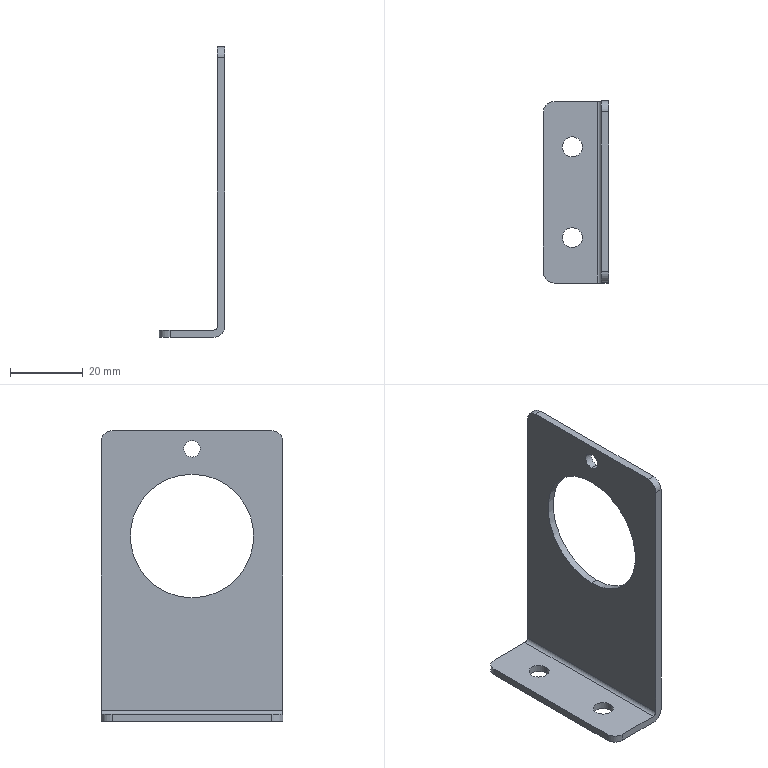Part | STEP file | ASND-0110-TPIM-069 | 1 solid | 22 faces | box 18 x 50 x 80 mm | volume 7556 mm3 | cylinder 14 | plane 8 | commonest cylinder face diameters 6 x5 5.5 x4 4.5 x2 34 x2 2 x1